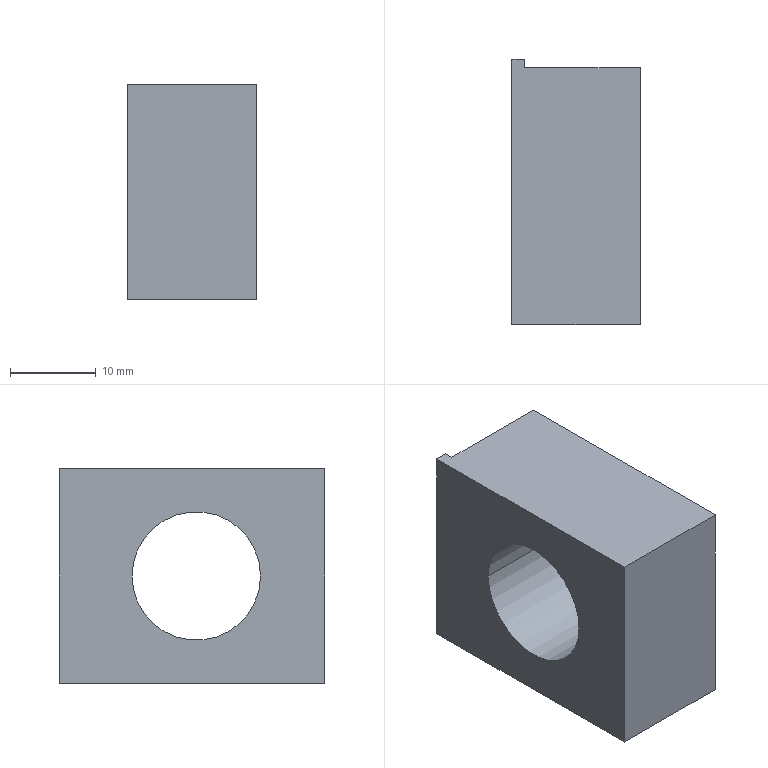Part | STEP file | 11-FG-B00511 | 1 solid | 22 faces | box 15 x 31 x 25 mm | volume 8369 mm3 | cylinder 8 | plane 8 | cone 6 | commonest cylinder face diameters 3.3 x6 15 x2
STEP:
#1=CARTESIAN_POINT('',(9.15,5.,10.1));
#2=VERTEX_POINT('',#1);
#3=CARTESIAN_POINT('',(5.85,5.,10.1));
#4=VERTEX_POINT('',#3);
#5=CARTESIAN_POINT('',(7.5,5.,10.1));
#6=DIRECTION('',(0.,0.,-1.));
#7=DIRECTION('',(-1.,0.,0.));
#8=AXIS2_PLACEMENT_3D('',#5,#6,#7);
#9=CIRCLE('',#8,1.65);
#10=EDGE_CURVE('',#2,#4,#9,.T.);
#11=ORIENTED_EDGE('',*,*,#10,.F.);
#12=CARTESIAN_POINT('',(9.15,5.,0.));
#13=VERTEX_POINT('',#12);
#14=CARTESIAN_POINT('',(9.15,5.,0.));
#15=DIRECTION('',(0.,0.,-1.));
#16=VECTOR('',#15,1000.);
#17=LINE('',#14,#16);
#18=EDGE_CURVE('',#2,#13,#17,.T.);
#19=ORIENTED_EDGE('',*,*,#18,.T.);
#20=CARTESIAN_POINT('',(5.85,5.,0.));
#21=VERTEX_POINT('',#20);
#22=CARTESIAN_POINT('',(7.5,5.,0.));
#23=DIRECTION('',(0.,0.,-1.));
#24=DIRECTION('',(-1.,0.,0.));
#25=AXIS2_PLACEMENT_3D('',#22,#23,#24);
#26=CIRCLE('',#25,1.65);
#27=EDGE_CURVE('',#13,#21,#26,.T.);
#28=ORIENTED_EDGE('',*,*,#27,.T.);
#29=CARTESIAN_POINT('',(5.85,5.,0.));
#30=DIRECTION('',(0.,0.,-1.));
#31=VECTOR('',#30,1000.);
#32=LINE('',#29,#31);
#33=EDGE_CURVE('',#4,#21,#32,.T.);
#34=ORIENTED_EDGE('',*,*,#33,.F.);
#35=EDGE_LOOP('',(#11,#19,#28,#34));
#36=FACE_OUTER_BOUND('',#35,.T.);
#37=CARTESIAN_POINT('',(7.5,5.,0.));
#38=DIRECTION('',(0.,0.,-1.));
#39=DIRECTION('',(-1.,0.,0.));
#40=AXIS2_PLACEMENT_3D('',#37,#38,#39);
#41=CYLINDRICAL_SURFACE('',#40,1.65);
#42=ADVANCED_FACE('',(#36),#41,.F.);
#43=CARTESIAN_POINT('',(7.5,5.,11.091));
#44=VERTEX_POINT('',#43);
#45=CARTESIAN_POINT('',(5.85,5.,10.1));
#46=DIRECTION('',(-0.8572,0.,-0.515));
#47=VECTOR('',#46,1000.);
#48=LINE('',#45,#47);
#49=EDGE_CURVE('',#44,#4,#48,.T.);
#50=ORIENTED_EDGE('',*,*,#49,.F.);
#51=CARTESIAN_POINT('',(9.15,5.,10.1));
#52=DIRECTION('',(0.8572,0.,-0.515));
#53=VECTOR('',#52,1000.);
#54=LINE('',#51,#53);
#55=EDGE_CURVE('',#44,#2,#54,.T.);
#56=ORIENTED_EDGE('',*,*,#55,.T.);
#57=ORIENTED_EDGE('',*,*,#10,.T.);
#58=EDGE_LOOP('',(#50,#56,#57));
#59=FACE_OUTER_BOUND('',#58,.T.);
#60=CARTESIAN_POINT('',(7.5,5.,10.1));
#61=DIRECTION('',(0.,0.,-1.));
#62=DIRECTION('',(-1.,0.,0.));
#63=AXIS2_PLACEMENT_3D('',#60,#61,#62);
#64=CONICAL_SURFACE('',#63,1.65,1.03);
#65=ADVANCED_FACE('',(#59),#64,.F.);
#66=CARTESIAN_POINT('',(6.5,19.9,3.35));
#67=VERTEX_POINT('',#66);
#68=CARTESIAN_POINT('',(6.5,19.9,6.65));
#69=VERTEX_POINT('',#68);
#70=CARTESIAN_POINT('',(6.5,19.9,5.));
#71=DIRECTION('',(0.,1.,0.));
#72=DIRECTION('',(0.,0.,1.));
#73=AXIS2_PLACEMENT_3D('',#70,#71,#72);
#74=CIRCLE('',#73,1.65);
#75=EDGE_CURVE('',#67,#69,#74,.T.);
#76=ORIENTED_EDGE('',*,*,#75,.F.);
#77=CARTESIAN_POINT('',(6.5,30.,3.35));
#78=VERTEX_POINT('',#77);
#79=CARTESIAN_POINT('',(6.5,30.,3.35));
#80=DIRECTION('',(0.,1.,0.));
#81=VECTOR('',#80,1000.);
#82=LINE('',#79,#81);
#83=EDGE_CURVE('',#67,#78,#82,.T.);
#84=ORIENTED_EDGE('',*,*,#83,.T.);
#85=CARTESIAN_POINT('',(6.5,30.,6.65));
#86=VERTEX_POINT('',#85);
#87=CARTESIAN_POINT('',(6.5,30.,5.));
#88=DIRECTION('',(0.,1.,0.));
#89=DIRECTION('',(0.,0.,1.));
#90=AXIS2_PLACEMENT_3D('',#87,#88,#89);
#91=CIRCLE('',#90,1.65);
#92=EDGE_CURVE('',#78,#86,#91,.T.);
#93=ORIENTED_EDGE('',*,*,#92,.T.);
#94=CARTESIAN_POINT('',(6.5,30.,6.65));
#95=DIRECTION('',(0.,1.,0.));
#96=VECTOR('',#95,1000.);
#97=LINE('',#94,#96);
#98=EDGE_CURVE('',#69,#86,#97,.T.);
#99=ORIENTED_EDGE('',*,*,#98,.F.);
#100=EDGE_LOOP('',(#76,#84,#93,#99));
#101=FACE_OUTER_BOUND('',#100,.T.);
#102=CARTESIAN_POINT('',(6.5,30.,5.));
#103=DIRECTION('',(0.,1.,0.));
#104=DIRECTION('',(0.,0.,1.));
#105=AXIS2_PLACEMENT_3D('',#102,#103,#104);
#106=CYLINDRICAL_SURFACE('',#105,1.65);
#107=ADVANCED_FACE('',(#101),#106,.F.);
#108=CARTESIAN_POINT('',(6.5,18.909,5.));
#109=VERTEX_POINT('',#108);
#110=CARTESIAN_POINT('',(6.5,19.9,6.65));
#111=DIRECTION('',(0.,0.515,0.8572));
#112=VECTOR('',#111,1000.);
#113=LINE('',#110,#112);
#114=EDGE_CURVE('',#109,#69,#113,.T.);
#115=ORIENTED_EDGE('',*,*,#114,.F.);
#116=CARTESIAN_POINT('',(6.5,19.9,3.35));
#117=DIRECTION('',(0.,0.515,-0.8572));
#118=VECTOR('',#117,1000.);
#119=LINE('',#116,#118);
#120=EDGE_CURVE('',#109,#67,#119,.T.);
#121=ORIENTED_EDGE('',*,*,#120,.T.);
#122=ORIENTED_EDGE('',*,*,#75,.T.);
#123=EDGE_LOOP('',(#115,#121,#122));
#124=FACE_OUTER_BOUND('',#123,.T.);
#125=CARTESIAN_POINT('',(6.5,19.9,5.));
#126=DIRECTION('',(0.,1.,0.));
#127=DIRECTION('',(0.,0.,1.));
#128=AXIS2_PLACEMENT_3D('',#125,#126,#127);
#129=CONICAL_SURFACE('',#128,1.65,1.03);
#130=ADVANCED_FACE('',(#124),#129,.F.);
#131=CARTESIAN_POINT('',(6.5,19.9,18.35));
#132=VERTEX_POINT('',#131);
#133=CARTESIAN_POINT('',(6.5,19.9,21.65));
#134=VERTEX_POINT('',#133);
#135=CARTESIAN_POINT('',(6.5,19.9,20.));
#136=DIRECTION('',(0.,1.,0.));
#137=DIRECTION('',(0.,0.,1.));
#138=AXIS2_PLACEMENT_3D('',#135,#136,#137);
#139=CIRCLE('',#138,1.65);
#140=EDGE_CURVE('',#132,#134,#139,.T.);
#141=ORIENTED_EDGE('',*,*,#140,.F.);
#142=CARTESIAN_POINT('',(6.5,30.,18.35));
#143=VERTEX_POINT('',#142);
#144=CARTESIAN_POINT('',(6.5,30.,18.35));
#145=DIRECTION('',(0.,1.,0.));
#146=VECTOR('',#145,1000.);
#147=LINE('',#144,#146);
#148=EDGE_CURVE('',#132,#143,#147,.T.);
#149=ORIENTED_EDGE('',*,*,#148,.T.);
#150=CARTESIAN_POINT('',(6.5,30.,21.65));
#151=VERTEX_POINT('',#150);
#152=CARTESIAN_POINT('',(6.5,30.,20.));
#153=DIRECTION('',(0.,1.,0.));
#154=DIRECTION('',(0.,0.,1.));
#155=AXIS2_PLACEMENT_3D('',#152,#153,#154);
#156=CIRCLE('',#155,1.65);
#157=EDGE_CURVE('',#143,#151,#156,.T.);
#158=ORIENTED_EDGE('',*,*,#157,.T.);
#159=CARTESIAN_POINT('',(6.5,30.,21.65));
#160=DIRECTION('',(0.,1.,0.));
#161=VECTOR('',#160,1000.);
#162=LINE('',#159,#161);
#163=EDGE_CURVE('',#134,#151,#162,.T.);
#164=ORIENTED_EDGE('',*,*,#163,.F.);
#165=EDGE_LOOP('',(#141,#149,#158,#164));
#166=FACE_OUTER_BOUND('',#165,.T.);
#167=CARTESIAN_POINT('',(6.5,30.,20.));
#168=DIRECTION('',(0.,1.,0.));
#169=DIRECTION('',(0.,0.,1.));
#170=AXIS2_PLACEMENT_3D('',#167,#168,#169);
#171=CYLINDRICAL_SURFACE('',#170,1.65);
#172=ADVANCED_FACE('',(#166),#171,.F.);
#173=CARTESIAN_POINT('',(6.5,18.909,20.));
#174=VERTEX_POINT('',#173);
#175=CARTESIAN_POINT('',(6.5,19.9,21.65));
#176=DIRECTION('',(0.,0.515,0.8572));
#177=VECTOR('',#176,1000.);
#178=LINE('',#175,#177);
#179=EDGE_CURVE('',#174,#134,#178,.T.);
#180=ORIENTED_EDGE('',*,*,#179,.F.);
#181=CARTESIAN_POINT('',(6.5,19.9,18.35));
#182=DIRECTION('',(0.,0.515,-0.8572));
#183=VECTOR('',#182,1000.);
#184=LINE('',#181,#183);
#185=EDGE_CURVE('',#174,#132,#184,.T.);
#186=ORIENTED_EDGE('',*,*,#185,.T.);
#187=ORIENTED_EDGE('',*,*,#140,.T.);
#188=EDGE_LOOP('',(#180,#186,#187));
#189=FACE_OUTER_BOUND('',#188,.T.);
#190=CARTESIAN_POINT('',(6.5,19.9,20.));
#191=DIRECTION('',(0.,1.,0.));
#192=DIRECTION('',(0.,0.,1.));
#193=AXIS2_PLACEMENT_3D('',#190,#191,#192);
#194=CONICAL_SURFACE('',#193,1.65,1.03);
#195=ADVANCED_FACE('',(#189),#194,.F.);
#196=CARTESIAN_POINT('',(15.,22.5,12.5));
#197=VERTEX_POINT('',#196);
#198=CARTESIAN_POINT('',(15.,7.5,12.5));
#199=VERTEX_POINT('',#198);
#200=CARTESIAN_POINT('',(15.,15.,12.5));
#201=DIRECTION('',(-1.,0.,0.));
#202=DIRECTION('',(0.,-1.,0.));
#203=AXIS2_PLACEMENT_3D('',#200,#201,#202);
#204=CIRCLE('',#203,7.5);
#205=EDGE_CURVE('',#197,#199,#204,.T.);
#206=ORIENTED_EDGE('',*,*,#205,.F.);
#207=CARTESIAN_POINT('',(0.,22.5,12.5));
#208=VERTEX_POINT('',#207);
#209=CARTESIAN_POINT('',(15.,22.5,12.5));
#210=DIRECTION('',(-1.,0.,0.));
#211=VECTOR('',#210,1000.);
#212=LINE('',#209,#211);
#213=EDGE_CURVE('',#197,#208,#212,.T.);
#214=ORIENTED_EDGE('',*,*,#213,.T.);
#215=CARTESIAN_POINT('',(0.,7.5,12.5));
#216=VERTEX_POINT('',#215);
#217=CARTESIAN_POINT('',(0.,15.,12.5));
#218=DIRECTION('',(-1.,0.,0.));
#219=DIRECTION('',(0.,-1.,0.));
#220=AXIS2_PLACEMENT_3D('',#217,#218,#219);
#221=CIRCLE('',#220,7.5);
#222=EDGE_CURVE('',#208,#216,#221,.T.);
#223=ORIENTED_EDGE('',*,*,#222,.T.);
#224=CARTESIAN_POINT('',(15.,7.5,12.5));
#225=DIRECTION('',(-1.,0.,0.));
#226=VECTOR('',#225,1000.);
#227=LINE('',#224,#226);
#228=EDGE_CURVE('',#199,#216,#227,.T.);
#229=ORIENTED_EDGE('',*,*,#228,.F.);
#230=EDGE_LOOP('',(#206,#214,#223,#229));
#231=FACE_OUTER_BOUND('',#230,.T.);
#232=CARTESIAN_POINT('',(15.,15.,12.5));
#233=DIRECTION('',(-1.,0.,0.));
#234=DIRECTION('',(0.,-1.,0.));
#235=AXIS2_PLACEMENT_3D('',#232,#233,#234);
#236=CYLINDRICAL_SURFACE('',#235,7.5);
#237=ADVANCED_FACE('',(#231),#236,.F.);
#238=CARTESIAN_POINT('',(6.5,30.,20.));
#239=DIRECTION('',(0.,1.,0.));
#240=DIRECTION('',(0.,0.,1.));
#241=AXIS2_PLACEMENT_3D('',#238,#239,#240);
#242=CIRCLE('',#241,1.65);
#243=EDGE_CURVE('',#151,#143,#242,.T.);
#244=ORIENTED_EDGE('',*,*,#243,.F.);
#245=ORIENTED_EDGE('',*,*,#157,.F.);
#246=EDGE_LOOP('',(#244,#245));
#247=FACE_BOUND('',#246,.T.);
#248=CARTESIAN_POINT('',(6.5,30.,5.));
#249=DIRECTION('',(0.,1.,0.));
#250=DIRECTION('',(0.,0.,1.));
#251=AXIS2_PLACEMENT_3D('',#248,#249,#250);
#252=CIRCLE('',#251,1.65);
#253=EDGE_CURVE('',#86,#78,#252,.T.);
#254=ORIENTED_EDGE('',*,*,#253,.F.);
#255=ORIENTED_EDGE('',*,*,#92,.F.);
#256=EDGE_LOOP('',(#254,#255));
#257=FACE_BOUND('',#256,.T.);
#258=CARTESIAN_POINT('',(1.5,30.,25.));
#259=VERTEX_POINT('',#258);
#260=CARTESIAN_POINT('',(1.5,30.,0.));
#261=VERTEX_POINT('',#260);
#262=CARTESIAN_POINT('',(1.5,30.,0.));
#263=DIRECTION('',(0.,0.,-1.));
#264=VECTOR('',#263,1000.);
#265=LINE('',#262,#264);
#266=EDGE_CURVE('',#259,#261,#265,.T.);
#267=ORIENTED_EDGE('',*,*,#266,.F.);
#268=CARTESIAN_POINT('',(15.,30.,25.));
#269=VERTEX_POINT('',#268);
#270=CARTESIAN_POINT('',(0.,30.,25.));
#271=DIRECTION('',(-1.,0.,0.));
#272=VECTOR('',#271,1000.);
#273=LINE('',#270,#272);
#274=EDGE_CURVE('',#269,#259,#273,.T.);
#275=ORIENTED_EDGE('',*,*,#274,.F.);
#276=CARTESIAN_POINT('',(15.,30.,0.));
#277=VERTEX_POINT('',#276);
#278=CARTESIAN_POINT('',(15.,30.,25.));
#279=DIRECTION('',(0.,0.,-1.));
#280=VECTOR('',#279,1000.);
#281=LINE('',#278,#280);
#282=EDGE_CURVE('',#269,#277,#281,.T.);
#283=ORIENTED_EDGE('',*,*,#282,.T.);
#284=CARTESIAN_POINT('',(0.,30.,0.));
#285=DIRECTION('',(-1.,0.,0.));
#286=VECTOR('',#285,1000.);
#287=LINE('',#284,#286);
#288=EDGE_CURVE('',#277,#261,#287,.T.);
#289=ORIENTED_EDGE('',*,*,#288,.T.);
#290=EDGE_LOOP('',(#267,#275,#283,#289));
#291=FACE_OUTER_BOUND('',#290,.T.);
#292=CARTESIAN_POINT('',(0.,30.,25.));
#293=DIRECTION('',(0.,-1.,0.));
#294=DIRECTION('',(0.,0.,-1.));
#295=AXIS2_PLACEMENT_3D('',#292,#293,#294);
#296=PLANE('',#295);
#297=ADVANCED_FACE('',(#247,#257,#291),#296,.F.);
#298=CARTESIAN_POINT('',(0.,15.,12.5));
#299=DIRECTION('',(-1.,0.,0.));
#300=DIRECTION('',(0.,-1.,0.));
#301=AXIS2_PLACEMENT_3D('',#298,#299,#300);
#302=CIRCLE('',#301,7.5);
#303=EDGE_CURVE('',#216,#208,#302,.T.);
#304=ORIENTED_EDGE('',*,*,#303,.F.);
#305=ORIENTED_EDGE('',*,*,#222,.F.);
#306=EDGE_LOOP('',(#304,#305));
#307=FACE_BOUND('',#306,.T.);
#308=CARTESIAN_POINT('',(0.,31.,0.));
#309=VERTEX_POINT('',#308);
#310=CARTESIAN_POINT('',(0.,0.,0.));
#311=VERTEX_POINT('',#310);
#312=CARTESIAN_POINT('',(0.,0.,0.));
#313=DIRECTION('',(0.,-1.,0.));
#314=VECTOR('',#313,1000.);
#315=LINE('',#312,#314);
#316=EDGE_CURVE('',#309,#311,#315,.T.);
#317=ORIENTED_EDGE('',*,*,#316,.T.);
#318=CARTESIAN_POINT('',(0.,0.,25.));
#319=VERTEX_POINT('',#318);
#320=CARTESIAN_POINT('',(0.,0.,25.));
#321=DIRECTION('',(0.,0.,-1.));
#322=VECTOR('',#321,1000.);
#323=LINE('',#320,#322);
#324=EDGE_CURVE('',#319,#311,#323,.T.);
#325=ORIENTED_EDGE('',*,*,#324,.F.);
#326=CARTESIAN_POINT('',(0.,31.,25.));
#327=VERTEX_POINT('',#326);
#328=CARTESIAN_POINT('',(0.,0.,25.));
#329=DIRECTION('',(0.,-1.,0.));
#330=VECTOR('',#329,1000.);
#331=LINE('',#328,#330);
#332=EDGE_CURVE('',#327,#319,#331,.T.);
#333=ORIENTED_EDGE('',*,*,#332,.F.);
#334=CARTESIAN_POINT('',(0.,31.,0.));
#335=DIRECTION('',(0.,0.,1.));
#336=VECTOR('',#335,1000.);
#337=LINE('',#334,#336);
#338=EDGE_CURVE('',#309,#327,#337,.T.);
#339=ORIENTED_EDGE('',*,*,#338,.F.);
#340=EDGE_LOOP('',(#317,#325,#333,#339));
#341=FACE_OUTER_BOUND('',#340,.T.);
#342=CARTESIAN_POINT('',(0.,0.,25.));
#343=DIRECTION('',(1.,0.,0.));
#344=DIRECTION('',(0.,1.,0.));
#345=AXIS2_PLACEMENT_3D('',#342,#343,#344);
#346=PLANE('',#345);
#347=ADVANCED_FACE('',(#307,#341),#346,.F.);
#348=CARTESIAN_POINT('',(15.,0.,0.));
#349=VERTEX_POINT('',#348);
#350=CARTESIAN_POINT('',(0.,0.,0.));
#351=DIRECTION('',(1.,0.,0.));
#352=VECTOR('',#351,1000.);
#353=LINE('',#350,#352);
#354=EDGE_CURVE('',#311,#349,#353,.T.);
#355=ORIENTED_EDGE('',*,*,#354,.T.);
#356=CARTESIAN_POINT('',(15.,0.,25.));
#357=VERTEX_POINT('',#356);
#358=CARTESIAN_POINT('',(15.,0.,25.));
#359=DIRECTION('',(0.,0.,-1.));
#360=VECTOR('',#359,1000.);
#361=LINE('',#358,#360);
#362=EDGE_CURVE('',#357,#349,#361,.T.);
#363=ORIENTED_EDGE('',*,*,#362,.F.);
#364=CARTESIAN_POINT('',(0.,0.,25.));
#365=DIRECTION('',(1.,0.,0.));
#366=VECTOR('',#365,1000.);
#367=LINE('',#364,#366);
#368=EDGE_CURVE('',#319,#357,#367,.T.);
#369=ORIENTED_EDGE('',*,*,#368,.F.);
#370=ORIENTED_EDGE('',*,*,#324,.T.);
#371=EDGE_LOOP('',(#355,#363,#369,#370));
#372=FACE_OUTER_BOUND('',#371,.T.);
#373=CARTESIAN_POINT('',(0.,0.,25.));
#374=DIRECTION('',(0.,1.,0.));
#375=DIRECTION('',(0.,0.,1.));
#376=AXIS2_PLACEMENT_3D('',#373,#374,#375);
#377=PLANE('',#376);
#378=ADVANCED_FACE('',(#372),#377,.F.);
#379=CARTESIAN_POINT('',(15.,15.,12.5));
#380=DIRECTION('',(-1.,0.,0.));
#381=DIRECTION('',(0.,-1.,0.));
#382=AXIS2_PLACEMENT_3D('',#379,#380,#381);
#383=CIRCLE('',#382,7.5);
#384=EDGE_CURVE('',#199,#197,#383,.T.);
#385=ORIENTED_EDGE('',*,*,#384,.T.);
#386=ORIENTED_EDGE('',*,*,#205,.T.);
#387=EDGE_LOOP('',(#385,#386));
#388=FACE_BOUND('',#387,.T.);
#389=CARTESIAN_POINT('',(15.,0.,0.));
#390=DIRECTION('',(0.,1.,0.));
#391=VECTOR('',#390,1000.);
#392=LINE('',#389,#391);
#393=EDGE_CURVE('',#349,#277,#392,.T.);
#394=ORIENTED_EDGE('',*,*,#393,.T.);
#395=ORIENTED_EDGE('',*,*,#282,.F.);
#396=CARTESIAN_POINT('',(15.,0.,25.));
#397=DIRECTION('',(0.,1.,0.));
#398=VECTOR('',#397,1000.);
#399=LINE('',#396,#398);
#400=EDGE_CURVE('',#357,#269,#399,.T.);
#401=ORIENTED_EDGE('',*,*,#400,.F.);
#402=ORIENTED_EDGE('',*,*,#362,.T.);
#403=EDGE_LOOP('',(#394,#395,#401,#402));
#404=FACE_OUTER_BOUND('',#403,.T.);
#405=CARTESIAN_POINT('',(15.,0.,25.));
#406=DIRECTION('',(-1.,0.,0.));
#407=DIRECTION('',(0.,-1.,0.));
#408=AXIS2_PLACEMENT_3D('',#405,#406,#407);
#409=PLANE('',#408);
#410=ADVANCED_FACE('',(#388,#404),#409,.F.);
#411=ORIENTED_EDGE('',*,*,#332,.T.);
#412=ORIENTED_EDGE('',*,*,#368,.T.);
#413=ORIENTED_EDGE('',*,*,#400,.T.);
#414=ORIENTED_EDGE('',*,*,#274,.T.);
#415=CARTESIAN_POINT('',(1.5,31.,25.));
#416=VERTEX_POINT('',#415);
#417=CARTESIAN_POINT('',(1.5,31.,25.));
#418=DIRECTION('',(0.,-1.,0.));
#419=VECTOR('',#418,1000.);
#420=LINE('',#417,#419);
#421=EDGE_CURVE('',#416,#259,#420,.T.);
#422=ORIENTED_EDGE('',*,*,#421,.F.);
#423=CARTESIAN_POINT('',(0.,31.,25.));
#424=DIRECTION('',(1.,0.,0.));
#425=VECTOR('',#424,1000.);
#426=LINE('',#423,#425);
#427=EDGE_CURVE('',#327,#416,#426,.T.);
#428=ORIENTED_EDGE('',*,*,#427,.F.);
#429=EDGE_LOOP('',(#411,#412,#413,#414,#422,#428));
#430=FACE_OUTER_BOUND('',#429,.T.);
#431=CARTESIAN_POINT('',(0.,30.,25.));
#432=DIRECTION('',(0.,0.,-1.));
#433=DIRECTION('',(-1.,0.,0.));
#434=AXIS2_PLACEMENT_3D('',#431,#432,#433);
#435=PLANE('',#434);
#436=ADVANCED_FACE('',(#430),#435,.F.);
#437=CARTESIAN_POINT('',(7.5,5.,0.));
#438=DIRECTION('',(0.,0.,-1.));
#439=DIRECTION('',(-1.,0.,0.));
#440=AXIS2_PLACEMENT_3D('',#437,#438,#439);
#441=CIRCLE('',#440,1.65);
#442=EDGE_CURVE('',#21,#13,#441,.T.);
#443=ORIENTED_EDGE('',*,*,#442,.F.);
#444=ORIENTED_EDGE('',*,*,#27,.F.);
#445=EDGE_LOOP('',(#443,#444));
#446=FACE_BOUND('',#445,.T.);
#447=ORIENTED_EDGE('',*,*,#316,.F.);
#448=CARTESIAN_POINT('',(1.5,31.,0.));
#449=VERTEX_POINT('',#448);
#450=CARTESIAN_POINT('',(0.,31.,0.));
#451=DIRECTION('',(-1.,0.,0.));
#452=VECTOR('',#451,1000.);
#453=LINE('',#450,#452);
#454=EDGE_CURVE('',#449,#309,#453,.T.);
#455=ORIENTED_EDGE('',*,*,#454,.F.);
#456=CARTESIAN_POINT('',(1.5,31.,0.));
#457=DIRECTION('',(0.,-1.,0.));
#458=VECTOR('',#457,1000.);
#459=LINE('',#456,#458);
#460=EDGE_CURVE('',#449,#261,#459,.T.);
#461=ORIENTED_EDGE('',*,*,#460,.T.);
#462=ORIENTED_EDGE('',*,*,#288,.F.);
#463=ORIENTED_EDGE('',*,*,#393,.F.);
#464=ORIENTED_EDGE('',*,*,#354,.F.);
#465=EDGE_LOOP('',(#447,#455,#461,#462,#463,#464));
#466=FACE_OUTER_BOUND('',#465,.T.);
#467=CARTESIAN_POINT('',(0.,30.,0.));
#468=DIRECTION('',(0.,0.,-1.));
#469=DIRECTION('',(-1.,0.,0.));
#470=AXIS2_PLACEMENT_3D('',#467,#468,#469);
#471=PLANE('',#470);
#472=ADVANCED_FACE('',(#446,#466),#471,.T.);
#473=ORIENTED_EDGE('',*,*,#213,.F.);
#474=ORIENTED_EDGE('',*,*,#384,.F.);
#475=ORIENTED_EDGE('',*,*,#228,.T.);
#476=ORIENTED_EDGE('',*,*,#303,.T.);
#477=EDGE_LOOP('',(#473,#474,#475,#476));
#478=FACE_OUTER_BOUND('',#477,.T.);
#479=CARTESIAN_POINT('',(15.,15.,12.5));
#480=DIRECTION('',(-1.,0.,0.));
#481=DIRECTION('',(0.,-1.,0.));
#482=AXIS2_PLACEMENT_3D('',#479,#480,#481);
#483=CYLINDRICAL_SURFACE('',#482,7.5);
#484=ADVANCED_FACE('',(#478),#483,.F.);
#485=ORIENTED_EDGE('',*,*,#185,.F.);
#486=ORIENTED_EDGE('',*,*,#179,.T.);
#487=CARTESIAN_POINT('',(6.5,19.9,20.));
#488=DIRECTION('',(0.,1.,0.));
#489=DIRECTION('',(0.,0.,1.));
#490=AXIS2_PLACEMENT_3D('',#487,#488,#489);
#491=CIRCLE('',#490,1.65);
#492=EDGE_CURVE('',#134,#132,#491,.T.);
#493=ORIENTED_EDGE('',*,*,#492,.T.);
#494=EDGE_LOOP('',(#485,#486,#493));
#495=FACE_OUTER_BOUND('',#494,.T.);
#496=CARTESIAN_POINT('',(6.5,19.9,20.));
#497=DIRECTION('',(0.,1.,0.));
#498=DIRECTION('',(0.,0.,1.));
#499=AXIS2_PLACEMENT_3D('',#496,#497,#498);
#500=CONICAL_SURFACE('',#499,1.65,1.03);
#501=ADVANCED_FACE('',(#495),#500,.F.);
#502=ORIENTED_EDGE('',*,*,#148,.F.);
#503=ORIENTED_EDGE('',*,*,#492,.F.);
#504=ORIENTED_EDGE('',*,*,#163,.T.);
#505=ORIENTED_EDGE('',*,*,#243,.T.);
#506=EDGE_LOOP('',(#502,#503,#504,#505));
#507=FACE_OUTER_BOUND('',#506,.T.);
#508=CARTESIAN_POINT('',(6.5,30.,20.));
#509=DIRECTION('',(0.,1.,0.));
#510=DIRECTION('',(0.,0.,1.));
#511=AXIS2_PLACEMENT_3D('',#508,#509,#510);
#512=CYLINDRICAL_SURFACE('',#511,1.65);
#513=ADVANCED_FACE('',(#507),#512,.F.);
#514=ORIENTED_EDGE('',*,*,#120,.F.);
#515=ORIENTED_EDGE('',*,*,#114,.T.);
#516=CARTESIAN_POINT('',(6.5,19.9,5.));
#517=DIRECTION('',(0.,1.,0.));
#518=DIRECTION('',(0.,0.,1.));
#519=AXIS2_PLACEMENT_3D('',#516,#517,#518);
#520=CIRCLE('',#519,1.65);
#521=EDGE_CURVE('',#69,#67,#520,.T.);
#522=ORIENTED_EDGE('',*,*,#521,.T.);
#523=EDGE_LOOP('',(#514,#515,#522));
#524=FACE_OUTER_BOUND('',#523,.T.);
#525=CARTESIAN_POINT('',(6.5,19.9,5.));
#526=DIRECTION('',(0.,1.,0.));
#527=DIRECTION('',(0.,0.,1.));
#528=AXIS2_PLACEMENT_3D('',#525,#526,#527);
#529=CONICAL_SURFACE('',#528,1.65,1.03);
#530=ADVANCED_FACE('',(#524),#529,.F.);
#531=ORIENTED_EDGE('',*,*,#83,.F.);
#532=ORIENTED_EDGE('',*,*,#521,.F.);
#533=ORIENTED_EDGE('',*,*,#98,.T.);
#534=ORIENTED_EDGE('',*,*,#253,.T.);
#535=EDGE_LOOP('',(#531,#532,#533,#534));
#536=FACE_OUTER_BOUND('',#535,.T.);
#537=CARTESIAN_POINT('',(6.5,30.,5.));
#538=DIRECTION('',(0.,1.,0.));
#539=DIRECTION('',(0.,0.,1.));
#540=AXIS2_PLACEMENT_3D('',#537,#538,#539);
#541=CYLINDRICAL_SURFACE('',#540,1.65);
#542=ADVANCED_FACE('',(#536),#541,.F.);
#543=ORIENTED_EDGE('',*,*,#266,.T.);
#544=ORIENTED_EDGE('',*,*,#460,.F.);
#545=CARTESIAN_POINT('',(1.5,31.,0.));
#546=DIRECTION('',(0.,0.,-1.));
#547=VECTOR('',#546,1000.);
#548=LINE('',#545,#547);
#549=EDGE_CURVE('',#416,#449,#548,.T.);
#550=ORIENTED_EDGE('',*,*,#549,.F.);
#551=ORIENTED_EDGE('',*,*,#421,.T.);
#552=EDGE_LOOP('',(#543,#544,#550,#551));
#553=FACE_OUTER_BOUND('',#552,.T.);
#554=CARTESIAN_POINT('',(1.5,31.,0.));
#555=DIRECTION('',(-1.,0.,0.));
#556=DIRECTION('',(0.,0.,1.));
#557=AXIS2_PLACEMENT_3D('',#554,#555,#556);
#558=PLANE('',#557);
#559=ADVANCED_FACE('',(#553),#558,.F.);
#560=ORIENTED_EDGE('',*,*,#338,.T.);
#561=ORIENTED_EDGE('',*,*,#427,.T.);
#562=ORIENTED_EDGE('',*,*,#549,.T.);
#563=ORIENTED_EDGE('',*,*,#454,.T.);
#564=EDGE_LOOP('',(#560,#561,#562,#563));
#565=FACE_OUTER_BOUND('',#564,.T.);
#566=CARTESIAN_POINT('',(0.,31.,25.));
#567=DIRECTION('',(0.,1.,0.));
#568=DIRECTION('',(0.,0.,1.));
#569=AXIS2_PLACEMENT_3D('',#566,#567,#568);
#570=PLANE('',#569);
#571=ADVANCED_FACE('',(#565),#570,.T.);
#572=ORIENTED_EDGE('',*,*,#55,.F.);
#573=ORIENTED_EDGE('',*,*,#49,.T.);
#574=CARTESIAN_POINT('',(7.5,5.,10.1));
#575=DIRECTION('',(0.,0.,-1.));
#576=DIRECTION('',(-1.,0.,0.));
#577=AXIS2_PLACEMENT_3D('',#574,#575,#576);
#578=CIRCLE('',#577,1.65);
#579=EDGE_CURVE('',#4,#2,#578,.T.);
#580=ORIENTED_EDGE('',*,*,#579,.T.);
#581=EDGE_LOOP('',(#572,#573,#580));
#582=FACE_OUTER_BOUND('',#581,.T.);
#583=CARTESIAN_POINT('',(7.5,5.,10.1));
#584=DIRECTION('',(0.,0.,-1.));
#585=DIRECTION('',(-1.,0.,0.));
#586=AXIS2_PLACEMENT_3D('',#583,#584,#585);
#587=CONICAL_SURFACE('',#586,1.65,1.03);
#588=ADVANCED_FACE('',(#582),#587,.F.);
#589=ORIENTED_EDGE('',*,*,#18,.F.);
#590=ORIENTED_EDGE('',*,*,#579,.F.);
#591=ORIENTED_EDGE('',*,*,#33,.T.);
#592=ORIENTED_EDGE('',*,*,#442,.T.);
#593=EDGE_LOOP('',(#589,#590,#591,#592));
#594=FACE_OUTER_BOUND('',#593,.T.);
#595=CARTESIAN_POINT('',(7.5,5.,0.));
#596=DIRECTION('',(0.,0.,-1.));
#597=DIRECTION('',(-1.,0.,0.));
#598=AXIS2_PLACEMENT_3D('',#595,#596,#597);
#599=CYLINDRICAL_SURFACE('',#598,1.65);
#600=ADVANCED_FACE('',(#594),#599,.F.);
#601=CLOSED_SHELL('',(#42,#65,#107,#130,#172,#195,#237,#297,#347,#378,#410,#436,#472,#484,#501,#513,#530,#542,#559,#571,#588,#600));
#602=MANIFOLD_SOLID_BREP('',#601);
#603=CARTESIAN_POINT('',(0.,0.,0.));
#604=DIRECTION('',(0.,0.,1.));
#605=DIRECTION('',(1.,0.,0.));
#606=AXIS2_PLACEMENT_3D('',#603,#604,#605);
#607=(LENGTH_UNIT()NAMED_UNIT(*)SI_UNIT(.MILLI.,.METRE.));
#608=UNCERTAINTY_MEASURE_WITH_UNIT(LENGTH_MEASURE(0.00001),#607,'','');
#609=(NAMED_UNIT(*)PLANE_ANGLE_UNIT()SI_UNIT($,.RADIAN.));
#610=(NAMED_UNIT(*)SI_UNIT($,.STERADIAN.)SOLID_ANGLE_UNIT());
#611=(GEOMETRIC_REPRESENTATION_CONTEXT(3)GLOBAL_UNCERTAINTY_ASSIGNED_CONTEXT((#608))GLOBAL_UNIT_ASSIGNED_CONTEXT((#607,#609,#610))REPRESENTATION_CONTEXT('',''));
#612=ADVANCED_BREP_SHAPE_REPRESENTATION('',(#602,#606),#611);